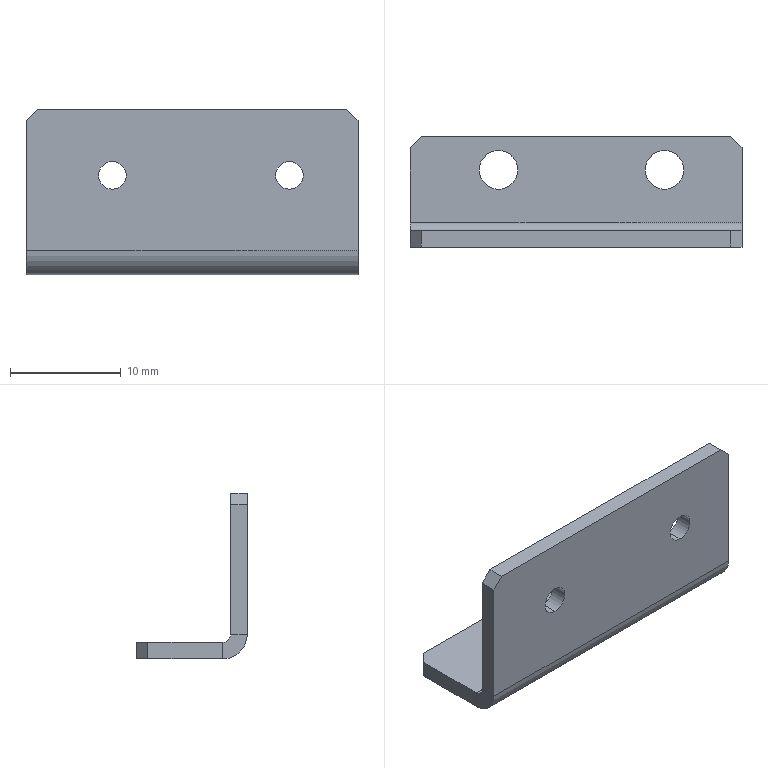Part | STEP file | PN_0035 BKT | 1 solid | 26 faces | box 30 x 10 x 15 mm | volume 982.198 mm3 | plane 16 | cylinder 10 | commonest cylinder face diameters 2.5 x4 3.5 x4 1.473 x1 4.473 x1